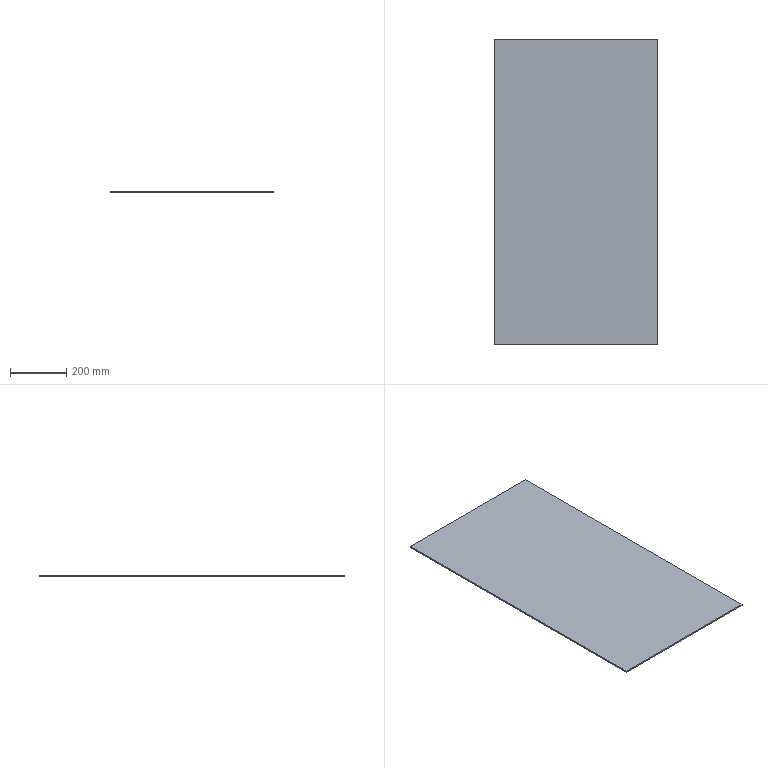Part | SolidWorks | features Extrusion 1, HoleWzd 1 | 1 solid | 6 faces | box 584 x 1091 x 5 mm | volume 3185720 mm3 | plane 6
STEP:
#1=CARTESIAN_POINT('',(292.,-545.5,0.));
#2=VERTEX_POINT('',#1);
#3=CARTESIAN_POINT('',(292.,545.5,0.));
#4=VERTEX_POINT('',#3);
#5=CARTESIAN_POINT('',(292.,545.5,0.));
#6=DIRECTION('',(0.,1.,0.));
#7=VECTOR('',#6,1000.);
#8=LINE('',#5,#7);
#9=EDGE_CURVE('',#2,#4,#8,.T.);
#10=ORIENTED_EDGE('',*,*,#9,.T.);
#11=CARTESIAN_POINT('',(292.,545.5,5.));
#12=VERTEX_POINT('',#11);
#13=CARTESIAN_POINT('',(292.,545.5,5.));
#14=DIRECTION('',(0.,0.,-1.));
#15=VECTOR('',#14,1000.);
#16=LINE('',#13,#15);
#17=EDGE_CURVE('',#12,#4,#16,.T.);
#18=ORIENTED_EDGE('',*,*,#17,.F.);
#19=CARTESIAN_POINT('',(292.,-545.5,5.));
#20=VERTEX_POINT('',#19);
#21=CARTESIAN_POINT('',(292.,545.5,5.));
#22=DIRECTION('',(0.,1.,0.));
#23=VECTOR('',#22,1000.);
#24=LINE('',#21,#23);
#25=EDGE_CURVE('',#20,#12,#24,.T.);
#26=ORIENTED_EDGE('',*,*,#25,.F.);
#27=CARTESIAN_POINT('',(292.,-545.5,5.));
#28=DIRECTION('',(0.,0.,-1.));
#29=VECTOR('',#28,1000.);
#30=LINE('',#27,#29);
#31=EDGE_CURVE('',#20,#2,#30,.T.);
#32=ORIENTED_EDGE('',*,*,#31,.T.);
#33=EDGE_LOOP('',(#10,#18,#26,#32));
#34=FACE_OUTER_BOUND('',#33,.T.);
#35=CARTESIAN_POINT('',(292.,545.5,5.));
#36=DIRECTION('',(-1.,0.,0.));
#37=DIRECTION('',(0.,-1.,0.));
#38=AXIS2_PLACEMENT_3D('',#35,#36,#37);
#39=PLANE('',#38);
#40=ADVANCED_FACE('',(#34),#39,.F.);
#41=CARTESIAN_POINT('',(-292.,545.5,0.));
#42=VERTEX_POINT('',#41);
#43=CARTESIAN_POINT('',(-292.,545.5,0.));
#44=DIRECTION('',(-1.,0.,0.));
#45=VECTOR('',#44,1000.);
#46=LINE('',#43,#45);
#47=EDGE_CURVE('',#4,#42,#46,.T.);
#48=ORIENTED_EDGE('',*,*,#47,.T.);
#49=CARTESIAN_POINT('',(-292.,545.5,5.));
#50=VERTEX_POINT('',#49);
#51=CARTESIAN_POINT('',(-292.,545.5,5.));
#52=DIRECTION('',(0.,0.,-1.));
#53=VECTOR('',#52,1000.);
#54=LINE('',#51,#53);
#55=EDGE_CURVE('',#50,#42,#54,.T.);
#56=ORIENTED_EDGE('',*,*,#55,.F.);
#57=CARTESIAN_POINT('',(-292.,545.5,5.));
#58=DIRECTION('',(-1.,0.,0.));
#59=VECTOR('',#58,1000.);
#60=LINE('',#57,#59);
#61=EDGE_CURVE('',#12,#50,#60,.T.);
#62=ORIENTED_EDGE('',*,*,#61,.F.);
#63=ORIENTED_EDGE('',*,*,#17,.T.);
#64=EDGE_LOOP('',(#48,#56,#62,#63));
#65=FACE_OUTER_BOUND('',#64,.T.);
#66=CARTESIAN_POINT('',(-292.,545.5,5.));
#67=DIRECTION('',(0.,-1.,0.));
#68=DIRECTION('',(0.,0.,-1.));
#69=AXIS2_PLACEMENT_3D('',#66,#67,#68);
#70=PLANE('',#69);
#71=ADVANCED_FACE('',(#65),#70,.F.);
#72=CARTESIAN_POINT('',(-292.,-545.5,0.));
#73=VERTEX_POINT('',#72);
#74=CARTESIAN_POINT('',(-292.,545.5,0.));
#75=DIRECTION('',(0.,-1.,0.));
#76=VECTOR('',#75,1000.);
#77=LINE('',#74,#76);
#78=EDGE_CURVE('',#42,#73,#77,.T.);
#79=ORIENTED_EDGE('',*,*,#78,.T.);
#80=CARTESIAN_POINT('',(-292.,-545.5,5.));
#81=VERTEX_POINT('',#80);
#82=CARTESIAN_POINT('',(-292.,-545.5,5.));
#83=DIRECTION('',(0.,0.,-1.));
#84=VECTOR('',#83,1000.);
#85=LINE('',#82,#84);
#86=EDGE_CURVE('',#81,#73,#85,.T.);
#87=ORIENTED_EDGE('',*,*,#86,.F.);
#88=CARTESIAN_POINT('',(-292.,545.5,5.));
#89=DIRECTION('',(0.,-1.,0.));
#90=VECTOR('',#89,1000.);
#91=LINE('',#88,#90);
#92=EDGE_CURVE('',#50,#81,#91,.T.);
#93=ORIENTED_EDGE('',*,*,#92,.F.);
#94=ORIENTED_EDGE('',*,*,#55,.T.);
#95=EDGE_LOOP('',(#79,#87,#93,#94));
#96=FACE_OUTER_BOUND('',#95,.T.);
#97=CARTESIAN_POINT('',(-292.,545.5,5.));
#98=DIRECTION('',(1.,0.,0.));
#99=DIRECTION('',(0.,1.,0.));
#100=AXIS2_PLACEMENT_3D('',#97,#98,#99);
#101=PLANE('',#100);
#102=ADVANCED_FACE('',(#96),#101,.F.);
#103=CARTESIAN_POINT('',(-292.,-545.5,0.));
#104=DIRECTION('',(1.,0.,0.));
#105=VECTOR('',#104,1000.);
#106=LINE('',#103,#105);
#107=EDGE_CURVE('',#73,#2,#106,.T.);
#108=ORIENTED_EDGE('',*,*,#107,.T.);
#109=ORIENTED_EDGE('',*,*,#31,.F.);
#110=CARTESIAN_POINT('',(-292.,-545.5,5.));
#111=DIRECTION('',(1.,0.,0.));
#112=VECTOR('',#111,1000.);
#113=LINE('',#110,#112);
#114=EDGE_CURVE('',#81,#20,#113,.T.);
#115=ORIENTED_EDGE('',*,*,#114,.F.);
#116=ORIENTED_EDGE('',*,*,#86,.T.);
#117=EDGE_LOOP('',(#108,#109,#115,#116));
#118=FACE_OUTER_BOUND('',#117,.T.);
#119=CARTESIAN_POINT('',(-292.,-545.5,5.));
#120=DIRECTION('',(0.,1.,0.));
#121=DIRECTION('',(0.,0.,1.));
#122=AXIS2_PLACEMENT_3D('',#119,#120,#121);
#123=PLANE('',#122);
#124=ADVANCED_FACE('',(#118),#123,.F.);
#125=ORIENTED_EDGE('',*,*,#25,.T.);
#126=ORIENTED_EDGE('',*,*,#61,.T.);
#127=ORIENTED_EDGE('',*,*,#92,.T.);
#128=ORIENTED_EDGE('',*,*,#114,.T.);
#129=EDGE_LOOP('',(#125,#126,#127,#128));
#130=FACE_OUTER_BOUND('',#129,.T.);
#131=CARTESIAN_POINT('',(0.,0.,5.));
#132=DIRECTION('',(0.,0.,1.));
#133=DIRECTION('',(1.,0.,0.));
#134=AXIS2_PLACEMENT_3D('',#131,#132,#133);
#135=PLANE('',#134);
#136=ADVANCED_FACE('',(#130),#135,.T.);
#137=ORIENTED_EDGE('',*,*,#9,.F.);
#138=ORIENTED_EDGE('',*,*,#107,.F.);
#139=ORIENTED_EDGE('',*,*,#78,.F.);
#140=ORIENTED_EDGE('',*,*,#47,.F.);
#141=EDGE_LOOP('',(#137,#138,#139,#140));
#142=FACE_OUTER_BOUND('',#141,.T.);
#143=CARTESIAN_POINT('',(0.,0.,0.));
#144=DIRECTION('',(0.,0.,1.));
#145=DIRECTION('',(1.,0.,0.));
#146=AXIS2_PLACEMENT_3D('',#143,#144,#145);
#147=PLANE('',#146);
#148=ADVANCED_FACE('',(#142),#147,.F.);
#149=CLOSED_SHELL('',(#40,#71,#102,#124,#136,#148));
#150=MANIFOLD_SOLID_BREP('',#149);
#151=CARTESIAN_POINT('',(0.,0.,0.));
#152=DIRECTION('',(0.,0.,1.));
#153=DIRECTION('',(1.,0.,0.));
#154=AXIS2_PLACEMENT_3D('',#151,#152,#153);
#155=(LENGTH_UNIT()NAMED_UNIT(*)SI_UNIT(.MILLI.,.METRE.));
#156=UNCERTAINTY_MEASURE_WITH_UNIT(LENGTH_MEASURE(0.00001),#155,'','');
#157=(NAMED_UNIT(*)PLANE_ANGLE_UNIT()SI_UNIT($,.RADIAN.));
#158=(NAMED_UNIT(*)SI_UNIT($,.STERADIAN.)SOLID_ANGLE_UNIT());
#159=(GEOMETRIC_REPRESENTATION_CONTEXT(3)GLOBAL_UNCERTAINTY_ASSIGNED_CONTEXT((#156))GLOBAL_UNIT_ASSIGNED_CONTEXT((#155,#157,#158))REPRESENTATION_CONTEXT('',''));
#160=ADVANCED_BREP_SHAPE_REPRESENTATION('',(#150,#154),#159);